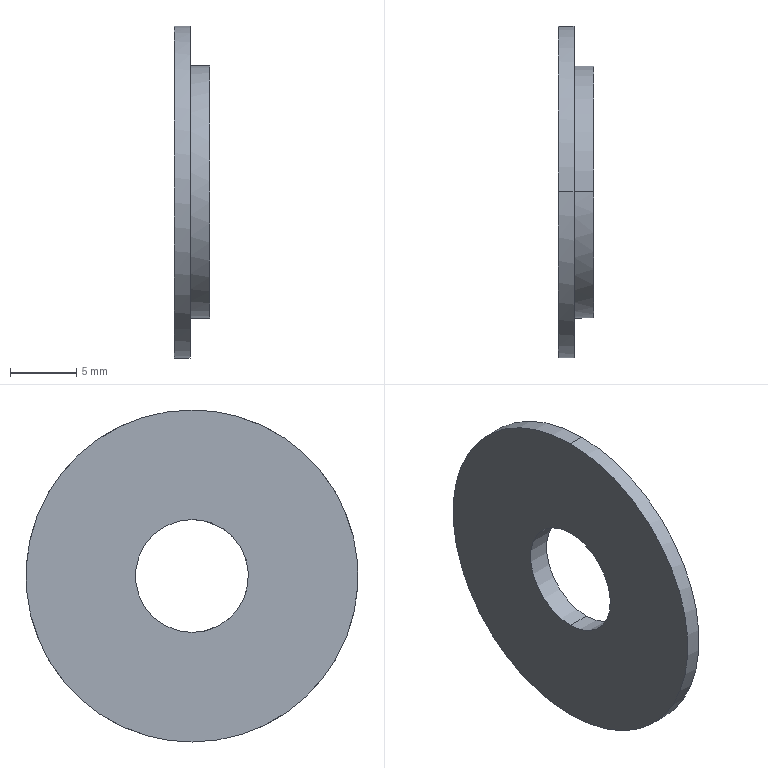Part | STEP file | 101000007604 | 1 solid | 12 faces | box 2.7 x 25 x 25 mm | volume 785.143 mm3 | cylinder 8 | plane 4 | commonest cylinder face diameters 8.5 x2 13 x2 19 x2 25 x2
STEP:
#1=CARTESIAN_POINT('',(9.259,0.,-6.5));
#2=VERTEX_POINT('',#1);
#3=CARTESIAN_POINT('',(9.259,0.,6.5));
#4=VERTEX_POINT('',#3);
#5=CARTESIAN_POINT('',(9.259,0.,-6.5));
#6=CARTESIAN_POINT('',(9.259,-1.021,-6.5));
#7=CARTESIAN_POINT('',(9.259,-2.042,-6.3));
#8=CARTESIAN_POINT('',(9.259,-3.01,-5.898));
#9=CARTESIAN_POINT('',(9.259,-4.738,-4.738));
#10=CARTESIAN_POINT('',(9.259,-5.898,-3.01));
#11=CARTESIAN_POINT('',(9.259,-6.3,-2.042));
#12=CARTESIAN_POINT('',(9.259,-6.7,0.));
#13=CARTESIAN_POINT('',(9.259,-6.3,2.042));
#14=CARTESIAN_POINT('',(9.259,-5.898,3.01));
#15=CARTESIAN_POINT('',(9.259,-4.738,4.738));
#16=CARTESIAN_POINT('',(9.259,-3.01,5.898));
#17=CARTESIAN_POINT('',(9.259,-2.042,6.3));
#18=CARTESIAN_POINT('',(9.259,-1.021,6.5));
#19=CARTESIAN_POINT('',(9.259,0.,6.5));
#20=B_SPLINE_CURVE_WITH_KNOTS('',5,(#5,#6,#7,#8,#9,#10,#11,#12,#13,#14,#15,#16,#17,#18,#19),.UNSPECIFIED.,.F.,.U.,(6,3,3,3,6),(-10.21,-5.105,0.,5.105,10.21),.UNSPECIFIED.);
#21=EDGE_CURVE('',#2,#4,#20,.T.);
#22=ORIENTED_EDGE('',*,*,#21,.F.);
#23=CARTESIAN_POINT('',(8.259,0.,-6.5));
#24=VERTEX_POINT('',#23);
#25=CARTESIAN_POINT('',(0.,0.,-6.5));
#26=DIRECTION('',(-1.,0.,0.));
#27=VECTOR('',#26,1.);
#28=LINE('',#25,#27);
#29=EDGE_CURVE('',#2,#24,#28,.T.);
#30=ORIENTED_EDGE('',*,*,#29,.T.);
#31=CARTESIAN_POINT('',(8.259,0.,6.5));
#32=VERTEX_POINT('',#31);
#33=CARTESIAN_POINT('',(8.259,0.,-6.5));
#34=CARTESIAN_POINT('',(8.259,-1.021,-6.5));
#35=CARTESIAN_POINT('',(8.259,-2.042,-6.3));
#36=CARTESIAN_POINT('',(8.259,-3.01,-5.898));
#37=CARTESIAN_POINT('',(8.259,-4.738,-4.738));
#38=CARTESIAN_POINT('',(8.259,-5.898,-3.01));
#39=CARTESIAN_POINT('',(8.259,-6.3,-2.042));
#40=CARTESIAN_POINT('',(8.259,-6.7,0.));
#41=CARTESIAN_POINT('',(8.259,-6.3,2.042));
#42=CARTESIAN_POINT('',(8.259,-5.898,3.01));
#43=CARTESIAN_POINT('',(8.259,-4.738,4.738));
#44=CARTESIAN_POINT('',(8.259,-3.01,5.898));
#45=CARTESIAN_POINT('',(8.259,-2.042,6.3));
#46=CARTESIAN_POINT('',(8.259,-1.021,6.5));
#47=CARTESIAN_POINT('',(8.259,0.,6.5));
#48=B_SPLINE_CURVE_WITH_KNOTS('',5,(#33,#34,#35,#36,#37,#38,#39,#40,#41,#42,#43,#44,#45,#46,#47),.UNSPECIFIED.,.F.,.U.,(6,3,3,3,6),(-10.21,-5.105,0.,5.105,10.21),.UNSPECIFIED.);
#49=EDGE_CURVE('',#24,#32,#48,.T.);
#50=ORIENTED_EDGE('',*,*,#49,.T.);
#51=CARTESIAN_POINT('',(0.,0.,6.5));
#52=DIRECTION('',(-1.,0.,0.));
#53=VECTOR('',#52,1.);
#54=LINE('',#51,#53);
#55=EDGE_CURVE('',#4,#32,#54,.T.);
#56=ORIENTED_EDGE('',*,*,#55,.F.);
#57=EDGE_LOOP('',(#22,#30,#50,#56));
#58=FACE_OUTER_BOUND('',#57,.T.);
#59=CARTESIAN_POINT('',(0.,0.,0.));
#60=DIRECTION('',(-1.,0.,0.));
#61=DIRECTION('',(0.,0.,-1.));
#62=AXIS2_PLACEMENT_3D('',#59,#60,#61);
#63=CYLINDRICAL_SURFACE('',#62,6.5);
#64=ADVANCED_FACE('',(#58),#63,.F.);
#65=CARTESIAN_POINT('',(9.259,0.,9.5));
#66=VERTEX_POINT('',#65);
#67=CARTESIAN_POINT('',(9.259,0.,-9.5));
#68=VERTEX_POINT('',#67);
#69=CARTESIAN_POINT('',(9.259,0.,0.));
#70=DIRECTION('',(-1.,0.,0.));
#71=AXIS2_PLACEMENT_3D('',#69,#70,$);
#72=CIRCLE('',#71,9.5);
#73=EDGE_CURVE('',#66,#68,#72,.T.);
#74=ORIENTED_EDGE('',*,*,#73,.F.);
#75=CARTESIAN_POINT('',(9.259,0.,0.));
#76=DIRECTION('',(-1.,0.,0.));
#77=AXIS2_PLACEMENT_3D('',#75,#76,$);
#78=CIRCLE('',#77,9.5);
#79=EDGE_CURVE('',#68,#66,#78,.T.);
#80=ORIENTED_EDGE('',*,*,#79,.F.);
#81=EDGE_LOOP('',(#74,#80));
#82=FACE_OUTER_BOUND('',#81,.T.);
#83=CARTESIAN_POINT('',(9.259,0.,0.));
#84=DIRECTION('',(-1.,0.,0.));
#85=AXIS2_PLACEMENT_3D('',#83,#84,$);
#86=CIRCLE('',#85,6.5);
#87=EDGE_CURVE('',#4,#2,#86,.T.);
#88=ORIENTED_EDGE('',*,*,#87,.T.);
#89=ORIENTED_EDGE('',*,*,#21,.T.);
#90=EDGE_LOOP('',(#88,#89));
#91=FACE_BOUND('',#90,.T.);
#92=CARTESIAN_POINT('',(9.259,9.5,0.));
#93=DIRECTION('',(-1.,0.,0.));
#94=DIRECTION('',(0.,0.,1.));
#95=AXIS2_PLACEMENT_3D('',#92,#93,#94);
#96=PLANE('',#95);
#97=ADVANCED_FACE('',(#82,#91),#96,.F.);
#98=ORIENTED_EDGE('',*,*,#29,.F.);
#99=ORIENTED_EDGE('',*,*,#87,.F.);
#100=ORIENTED_EDGE('',*,*,#55,.T.);
#101=CARTESIAN_POINT('',(8.259,0.,0.));
#102=DIRECTION('',(-1.,0.,0.));
#103=AXIS2_PLACEMENT_3D('',#101,#102,$);
#104=CIRCLE('',#103,6.5);
#105=EDGE_CURVE('',#32,#24,#104,.T.);
#106=ORIENTED_EDGE('',*,*,#105,.T.);
#107=EDGE_LOOP('',(#98,#99,#100,#106));
#108=FACE_OUTER_BOUND('',#107,.T.);
#109=CARTESIAN_POINT('',(0.,0.,0.));
#110=DIRECTION('',(-1.,0.,0.));
#111=DIRECTION('',(0.,0.,1.));
#112=AXIS2_PLACEMENT_3D('',#109,#110,#111);
#113=CYLINDRICAL_SURFACE('',#112,6.5);
#114=ADVANCED_FACE('',(#108),#113,.F.);
#115=ORIENTED_EDGE('',*,*,#105,.F.);
#116=ORIENTED_EDGE('',*,*,#49,.F.);
#117=EDGE_LOOP('',(#115,#116));
#118=FACE_OUTER_BOUND('',#117,.T.);
#119=CARTESIAN_POINT('',(8.259,0.,4.25));
#120=VERTEX_POINT('',#119);
#121=CARTESIAN_POINT('',(8.259,0.,-4.25));
#122=VERTEX_POINT('',#121);
#123=CARTESIAN_POINT('',(8.259,0.,0.));
#124=DIRECTION('',(-1.,0.,0.));
#125=AXIS2_PLACEMENT_3D('',#123,#124,$);
#126=CIRCLE('',#125,4.25);
#127=EDGE_CURVE('',#120,#122,#126,.T.);
#128=ORIENTED_EDGE('',*,*,#127,.T.);
#129=CARTESIAN_POINT('',(8.259,0.,0.));
#130=DIRECTION('',(-1.,0.,0.));
#131=AXIS2_PLACEMENT_3D('',#129,#130,$);
#132=CIRCLE('',#131,4.25);
#133=EDGE_CURVE('',#122,#120,#132,.T.);
#134=ORIENTED_EDGE('',*,*,#133,.T.);
#135=EDGE_LOOP('',(#128,#134));
#136=FACE_BOUND('',#135,.T.);
#137=CARTESIAN_POINT('',(8.259,6.5,0.));
#138=DIRECTION('',(-1.,0.,0.));
#139=DIRECTION('',(0.,0.,1.));
#140=AXIS2_PLACEMENT_3D('',#137,#138,#139);
#141=PLANE('',#140);
#142=ADVANCED_FACE('',(#118,#136),#141,.F.);
#143=ORIENTED_EDGE('',*,*,#73,.T.);
#144=CARTESIAN_POINT('',(7.759,0.,-9.5));
#145=VERTEX_POINT('',#144);
#146=CARTESIAN_POINT('',(0.,0.,-9.5));
#147=DIRECTION('',(-1.,0.,0.));
#148=VECTOR('',#147,1.);
#149=LINE('',#146,#148);
#150=EDGE_CURVE('',#68,#145,#149,.T.);
#151=ORIENTED_EDGE('',*,*,#150,.T.);
#152=CARTESIAN_POINT('',(7.759,0.,9.5));
#153=VERTEX_POINT('',#152);
#154=CARTESIAN_POINT('',(7.759,0.,0.));
#155=DIRECTION('',(-1.,0.,0.));
#156=AXIS2_PLACEMENT_3D('',#154,#155,$);
#157=CIRCLE('',#156,9.5);
#158=EDGE_CURVE('',#153,#145,#157,.T.);
#159=ORIENTED_EDGE('',*,*,#158,.F.);
#160=CARTESIAN_POINT('',(0.,0.,9.5));
#161=DIRECTION('',(-1.,0.,0.));
#162=VECTOR('',#161,1.);
#163=LINE('',#160,#162);
#164=EDGE_CURVE('',#66,#153,#163,.T.);
#165=ORIENTED_EDGE('',*,*,#164,.F.);
#166=EDGE_LOOP('',(#143,#151,#159,#165));
#167=FACE_OUTER_BOUND('',#166,.T.);
#168=CARTESIAN_POINT('',(0.,0.,0.));
#169=DIRECTION('',(-1.,0.,0.));
#170=DIRECTION('',(0.,0.,1.));
#171=AXIS2_PLACEMENT_3D('',#168,#169,#170);
#172=CYLINDRICAL_SURFACE('',#171,9.5);
#173=ADVANCED_FACE('',(#167),#172,.T.);
#174=ORIENTED_EDGE('',*,*,#150,.F.);
#175=ORIENTED_EDGE('',*,*,#79,.T.);
#176=ORIENTED_EDGE('',*,*,#164,.T.);
#177=CARTESIAN_POINT('',(7.759,0.,-9.5));
#178=CARTESIAN_POINT('',(7.759,-1.492,-9.5));
#179=CARTESIAN_POINT('',(7.759,-2.985,-9.207));
#180=CARTESIAN_POINT('',(7.759,-4.4,-8.621));
#181=CARTESIAN_POINT('',(7.759,-6.925,-6.925));
#182=CARTESIAN_POINT('',(7.759,-8.621,-4.4));
#183=CARTESIAN_POINT('',(7.759,-9.207,-2.985));
#184=CARTESIAN_POINT('',(7.759,-9.793,0.));
#185=CARTESIAN_POINT('',(7.759,-9.207,2.985));
#186=CARTESIAN_POINT('',(7.759,-8.621,4.4));
#187=CARTESIAN_POINT('',(7.759,-6.925,6.925));
#188=CARTESIAN_POINT('',(7.759,-4.4,8.621));
#189=CARTESIAN_POINT('',(7.759,-2.985,9.207));
#190=CARTESIAN_POINT('',(7.759,-1.492,9.5));
#191=CARTESIAN_POINT('',(7.759,0.,9.5));
#192=B_SPLINE_CURVE_WITH_KNOTS('',5,(#177,#178,#179,#180,#181,#182,#183,#184,#185,#186,#187,#188,#189,#190,#191),.UNSPECIFIED.,.F.,.U.,(6,3,3,3,6),(-14.923,-7.461,0.,7.461,14.923),.UNSPECIFIED.);
#193=EDGE_CURVE('',#145,#153,#192,.T.);
#194=ORIENTED_EDGE('',*,*,#193,.F.);
#195=EDGE_LOOP('',(#174,#175,#176,#194));
#196=FACE_OUTER_BOUND('',#195,.T.);
#197=CARTESIAN_POINT('',(0.,0.,0.));
#198=DIRECTION('',(-1.,0.,0.));
#199=DIRECTION('',(0.,0.,-1.));
#200=AXIS2_PLACEMENT_3D('',#197,#198,#199);
#201=CYLINDRICAL_SURFACE('',#200,9.5);
#202=ADVANCED_FACE('',(#196),#201,.T.);
#203=CARTESIAN_POINT('',(6.559,0.,-4.25));
#204=VERTEX_POINT('',#203);
#205=CARTESIAN_POINT('',(0.,0.,-4.25));
#206=DIRECTION('',(-1.,0.,0.));
#207=VECTOR('',#206,1.);
#208=LINE('',#205,#207);
#209=EDGE_CURVE('',#122,#204,#208,.T.);
#210=ORIENTED_EDGE('',*,*,#209,.F.);
#211=ORIENTED_EDGE('',*,*,#127,.F.);
#212=CARTESIAN_POINT('',(6.559,0.,4.25));
#213=VERTEX_POINT('',#212);
#214=CARTESIAN_POINT('',(0.,0.,4.25));
#215=DIRECTION('',(-1.,0.,0.));
#216=VECTOR('',#215,1.);
#217=LINE('',#214,#216);
#218=EDGE_CURVE('',#120,#213,#217,.T.);
#219=ORIENTED_EDGE('',*,*,#218,.T.);
#220=CARTESIAN_POINT('',(6.559,0.,0.));
#221=DIRECTION('',(-1.,0.,0.));
#222=AXIS2_PLACEMENT_3D('',#220,#221,$);
#223=CIRCLE('',#222,4.25);
#224=EDGE_CURVE('',#213,#204,#223,.T.);
#225=ORIENTED_EDGE('',*,*,#224,.T.);
#226=EDGE_LOOP('',(#210,#211,#219,#225));
#227=FACE_OUTER_BOUND('',#226,.T.);
#228=CARTESIAN_POINT('',(0.,0.,0.));
#229=DIRECTION('',(-1.,0.,0.));
#230=DIRECTION('',(0.,0.,1.));
#231=AXIS2_PLACEMENT_3D('',#228,#229,#230);
#232=CYLINDRICAL_SURFACE('',#231,4.25);
#233=ADVANCED_FACE('',(#227),#232,.F.);
#234=ORIENTED_EDGE('',*,*,#133,.F.);
#235=ORIENTED_EDGE('',*,*,#209,.T.);
#236=CARTESIAN_POINT('',(6.559,0.,-4.25));
#237=CARTESIAN_POINT('',(6.559,-0.6676,-4.25));
#238=CARTESIAN_POINT('',(6.559,-1.335,-4.119));
#239=CARTESIAN_POINT('',(6.559,-1.968,-3.857));
#240=CARTESIAN_POINT('',(6.559,-3.098,-3.098));
#241=CARTESIAN_POINT('',(6.559,-3.857,-1.968));
#242=CARTESIAN_POINT('',(6.559,-4.119,-1.335));
#243=CARTESIAN_POINT('',(6.559,-4.381,0.));
#244=CARTESIAN_POINT('',(6.559,-4.119,1.335));
#245=CARTESIAN_POINT('',(6.559,-3.857,1.968));
#246=CARTESIAN_POINT('',(6.559,-3.098,3.098));
#247=CARTESIAN_POINT('',(6.559,-1.968,3.857));
#248=CARTESIAN_POINT('',(6.559,-1.335,4.119));
#249=CARTESIAN_POINT('',(6.559,-0.6676,4.25));
#250=CARTESIAN_POINT('',(6.559,0.,4.25));
#251=B_SPLINE_CURVE_WITH_KNOTS('',5,(#236,#237,#238,#239,#240,#241,#242,#243,#244,#245,#246,#247,#248,#249,#250),.UNSPECIFIED.,.F.,.U.,(6,3,3,3,6),(-6.676,-3.338,0.,3.338,6.676),.UNSPECIFIED.);
#252=EDGE_CURVE('',#204,#213,#251,.T.);
#253=ORIENTED_EDGE('',*,*,#252,.T.);
#254=ORIENTED_EDGE('',*,*,#218,.F.);
#255=EDGE_LOOP('',(#234,#235,#253,#254));
#256=FACE_OUTER_BOUND('',#255,.T.);
#257=CARTESIAN_POINT('',(0.,0.,0.));
#258=DIRECTION('',(-1.,0.,0.));
#259=DIRECTION('',(0.,0.,-1.));
#260=AXIS2_PLACEMENT_3D('',#257,#258,#259);
#261=CYLINDRICAL_SURFACE('',#260,4.25);
#262=ADVANCED_FACE('',(#256),#261,.F.);
#263=CARTESIAN_POINT('',(7.759,0.,12.5));
#264=VERTEX_POINT('',#263);
#265=CARTESIAN_POINT('',(7.759,0.,-12.5));
#266=VERTEX_POINT('',#265);
#267=CARTESIAN_POINT('',(7.759,0.,0.));
#268=DIRECTION('',(-1.,0.,0.));
#269=AXIS2_PLACEMENT_3D('',#267,#268,$);
#270=CIRCLE('',#269,12.5);
#271=EDGE_CURVE('',#264,#266,#270,.T.);
#272=ORIENTED_EDGE('',*,*,#271,.F.);
#273=CARTESIAN_POINT('',(7.759,0.,0.));
#274=DIRECTION('',(-1.,0.,0.));
#275=AXIS2_PLACEMENT_3D('',#273,#274,$);
#276=CIRCLE('',#275,12.5);
#277=EDGE_CURVE('',#266,#264,#276,.T.);
#278=ORIENTED_EDGE('',*,*,#277,.F.);
#279=EDGE_LOOP('',(#272,#278));
#280=FACE_OUTER_BOUND('',#279,.T.);
#281=ORIENTED_EDGE('',*,*,#158,.T.);
#282=ORIENTED_EDGE('',*,*,#193,.T.);
#283=EDGE_LOOP('',(#281,#282));
#284=FACE_BOUND('',#283,.T.);
#285=CARTESIAN_POINT('',(7.759,12.5,0.));
#286=DIRECTION('',(-1.,0.,0.));
#287=DIRECTION('',(0.,0.,1.));
#288=AXIS2_PLACEMENT_3D('',#285,#286,#287);
#289=PLANE('',#288);
#290=ADVANCED_FACE('',(#280,#284),#289,.F.);
#291=CARTESIAN_POINT('',(6.559,0.,12.5));
#292=VERTEX_POINT('',#291);
#293=CARTESIAN_POINT('',(6.559,0.,-12.5));
#294=VERTEX_POINT('',#293);
#295=CARTESIAN_POINT('',(6.559,0.,12.5));
#296=CARTESIAN_POINT('',(6.559,1.212,12.5));
#297=CARTESIAN_POINT('',(6.559,2.425,12.353));
#298=CARTESIAN_POINT('',(6.559,3.614,12.059));
#299=CARTESIAN_POINT('',(6.559,5.896,11.189));
#300=CARTESIAN_POINT('',(6.559,7.904,9.798));
#301=CARTESIAN_POINT('',(6.559,8.819,8.984));
#302=CARTESIAN_POINT('',(6.559,10.432,7.15));
#303=CARTESIAN_POINT('',(6.559,11.56,4.984));
#304=CARTESIAN_POINT('',(6.559,11.99,3.837));
#305=CARTESIAN_POINT('',(6.559,12.562,1.462));
#306=CARTESIAN_POINT('',(6.559,12.551,-0.9804));
#307=CARTESIAN_POINT('',(6.559,12.396,-2.195));
#308=CARTESIAN_POINT('',(6.559,11.795,-4.563));
#309=CARTESIAN_POINT('',(6.559,10.646,-6.718));
#310=CARTESIAN_POINT('',(6.559,9.943,-7.721));
#311=CARTESIAN_POINT('',(6.559,8.308,-9.535));
#312=CARTESIAN_POINT('',(6.559,6.287,-10.907));
#313=CARTESIAN_POINT('',(6.559,5.197,-11.466));
#314=CARTESIAN_POINT('',(6.559,3.503,-12.089));
#315=CARTESIAN_POINT('',(6.559,1.736,-12.399));
#316=CARTESIAN_POINT('',(6.559,1.159,-12.466));
#317=CARTESIAN_POINT('',(6.559,0.5794,-12.5));
#318=CARTESIAN_POINT('',(6.559,0.,-12.5));
#319=B_SPLINE_CURVE_WITH_KNOTS('',5,(#295,#296,#297,#298,#299,#300,#301,#302,#303,#304,#305,#306,#307,#308,#309,#310,#311,#312,#313,#314,#315,#316,#317,#318),.UNSPECIFIED.,.F.,.U.,(6,3,3,3,3,3,3,6),(0.,8.573,17.146,25.719,34.293,42.866,51.439,55.536),.UNSPECIFIED.);
#320=EDGE_CURVE('',#292,#294,#319,.T.);
#321=ORIENTED_EDGE('',*,*,#320,.T.);
#322=CARTESIAN_POINT('',(6.559,0.,-12.5));
#323=CARTESIAN_POINT('',(6.559,-1.212,-12.5));
#324=CARTESIAN_POINT('',(6.559,-2.425,-12.353));
#325=CARTESIAN_POINT('',(6.559,-3.614,-12.059));
#326=CARTESIAN_POINT('',(6.559,-5.896,-11.189));
#327=CARTESIAN_POINT('',(6.559,-7.904,-9.798));
#328=CARTESIAN_POINT('',(6.559,-8.819,-8.984));
#329=CARTESIAN_POINT('',(6.559,-10.432,-7.15));
#330=CARTESIAN_POINT('',(6.559,-11.56,-4.984));
#331=CARTESIAN_POINT('',(6.559,-11.99,-3.837));
#332=CARTESIAN_POINT('',(6.559,-12.562,-1.462));
#333=CARTESIAN_POINT('',(6.559,-12.551,0.9804));
#334=CARTESIAN_POINT('',(6.559,-12.396,2.195));
#335=CARTESIAN_POINT('',(6.559,-11.795,4.563));
#336=CARTESIAN_POINT('',(6.559,-10.646,6.718));
#337=CARTESIAN_POINT('',(6.559,-9.943,7.721));
#338=CARTESIAN_POINT('',(6.559,-8.308,9.535));
#339=CARTESIAN_POINT('',(6.559,-6.287,10.907));
#340=CARTESIAN_POINT('',(6.559,-5.197,11.466));
#341=CARTESIAN_POINT('',(6.559,-3.503,12.089));
#342=CARTESIAN_POINT('',(6.559,-1.736,12.399));
#343=CARTESIAN_POINT('',(6.559,-1.159,12.466));
#344=CARTESIAN_POINT('',(6.559,-0.5794,12.5));
#345=CARTESIAN_POINT('',(6.559,0.,12.5));
#346=B_SPLINE_CURVE_WITH_KNOTS('',5,(#322,#323,#324,#325,#326,#327,#328,#329,#330,#331,#332,#333,#334,#335,#336,#337,#338,#339,#340,#341,#342,#343,#344,#345),.UNSPECIFIED.,.F.,.U.,(6,3,3,3,3,3,3,6),(0.,8.573,17.146,25.719,34.293,42.866,51.439,55.536),.UNSPECIFIED.);
#347=EDGE_CURVE('',#294,#292,#346,.T.);
#348=ORIENTED_EDGE('',*,*,#347,.T.);
#349=EDGE_LOOP('',(#321,#348));
#350=FACE_OUTER_BOUND('',#349,.T.);
#351=ORIENTED_EDGE('',*,*,#224,.F.);
#352=ORIENTED_EDGE('',*,*,#252,.F.);
#353=EDGE_LOOP('',(#351,#352));
#354=FACE_BOUND('',#353,.T.);
#355=CARTESIAN_POINT('',(6.559,4.25,0.));
#356=DIRECTION('',(1.,0.,0.));
#357=DIRECTION('',(0.,0.,-1.));
#358=AXIS2_PLACEMENT_3D('',#355,#356,#357);
#359=PLANE('',#358);
#360=ADVANCED_FACE('',(#350,#354),#359,.F.);
#361=ORIENTED_EDGE('',*,*,#271,.T.);
#362=CARTESIAN_POINT('',(0.,0.,-12.5));
#363=DIRECTION('',(-1.,0.,0.));
#364=VECTOR('',#363,1.);
#365=LINE('',#362,#364);
#366=EDGE_CURVE('',#266,#294,#365,.T.);
#367=ORIENTED_EDGE('',*,*,#366,.T.);
#368=ORIENTED_EDGE('',*,*,#320,.F.);
#369=CARTESIAN_POINT('',(0.,0.,12.5));
#370=DIRECTION('',(-1.,0.,0.));
#371=VECTOR('',#370,1.);
#372=LINE('',#369,#371);
#373=EDGE_CURVE('',#264,#292,#372,.T.);
#374=ORIENTED_EDGE('',*,*,#373,.F.);
#375=EDGE_LOOP('',(#361,#367,#368,#374));
#376=FACE_OUTER_BOUND('',#375,.T.);
#377=CARTESIAN_POINT('',(0.,0.,0.));
#378=DIRECTION('',(-1.,0.,0.));
#379=DIRECTION('',(0.,0.,1.));
#380=AXIS2_PLACEMENT_3D('',#377,#378,#379);
#381=CYLINDRICAL_SURFACE('',#380,12.5);
#382=ADVANCED_FACE('',(#376),#381,.T.);
#383=ORIENTED_EDGE('',*,*,#366,.F.);
#384=ORIENTED_EDGE('',*,*,#277,.T.);
#385=ORIENTED_EDGE('',*,*,#373,.T.);
#386=ORIENTED_EDGE('',*,*,#347,.F.);
#387=EDGE_LOOP('',(#383,#384,#385,#386));
#388=FACE_OUTER_BOUND('',#387,.T.);
#389=CARTESIAN_POINT('',(0.,0.,0.));
#390=DIRECTION('',(-1.,0.,0.));
#391=DIRECTION('',(0.,0.,-1.));
#392=AXIS2_PLACEMENT_3D('',#389,#390,#391);
#393=CYLINDRICAL_SURFACE('',#392,12.5);
#394=ADVANCED_FACE('',(#388),#393,.T.);
#395=CLOSED_SHELL('',(#64,#97,#114,#142,#173,#202,#233,#262,#290,#360,#382,#394));
#396=MANIFOLD_SOLID_BREP('',#395);
#397=(LENGTH_UNIT()NAMED_UNIT(*)SI_UNIT(.MILLI.,.METRE.));
#398=UNCERTAINTY_MEASURE_WITH_UNIT(LENGTH_MEASURE(0.005),#397,'','');
#399=(NAMED_UNIT(*)PLANE_ANGLE_UNIT()SI_UNIT($,.RADIAN.));
#400=(NAMED_UNIT(*)SI_UNIT($,.STERADIAN.)SOLID_ANGLE_UNIT());
#401=(GEOMETRIC_REPRESENTATION_CONTEXT(3)GLOBAL_UNCERTAINTY_ASSIGNED_CONTEXT((#398))GLOBAL_UNIT_ASSIGNED_CONTEXT((#397,#399,#400))REPRESENTATION_CONTEXT('',''));
#402=ADVANCED_BREP_SHAPE_REPRESENTATION('',(#396),#401);